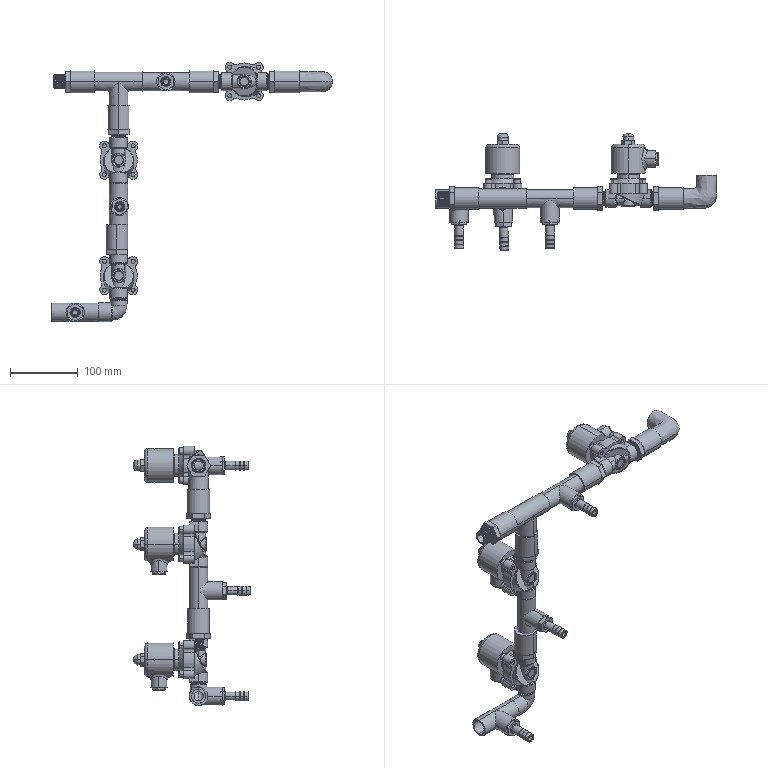Part | SolidWorks | features CompositeCurve 4 | 49 solids | 1644 faces | box 415.889 x 172.793 x 383.815 mm | volume 846980 mm3 | cylinder 558 | plane 425 | cone 396 | spline 179 | torus 86 | commonest cylinder face diameters 19.583 x120 18.5 x111 45 x51 10 x48 13.868 x31 6 x24